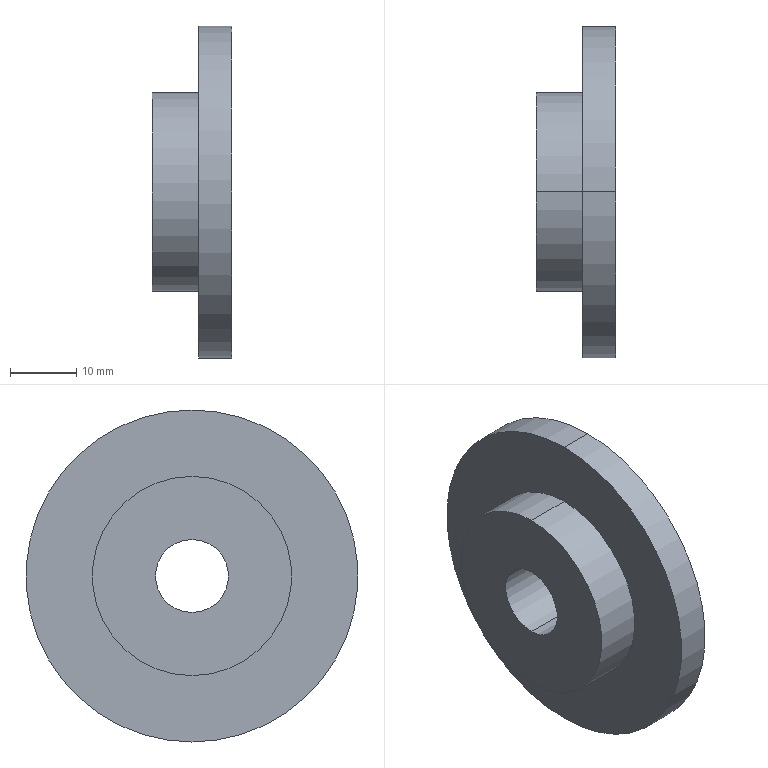Part | SolidWorks | features ICE 1, Revolution 1 | 1 solid | 9 faces | box 12 x 50 x 50 mm | volume 13625 mm3 | cylinder 6 | plane 3 | commonest cylinder face diameters 11 x2 30 x2 50 x2
STEP:
#1=CARTESIAN_POINT('',(0.,0.,5.5));
#2=VERTEX_POINT('',#1);
#3=CARTESIAN_POINT('',(0.,0.,-5.5));
#4=VERTEX_POINT('',#3);
#5=CARTESIAN_POINT('',(0.,0.,0.));
#6=DIRECTION('',(1.,0.,0.));
#7=DIRECTION('',(0.,0.,-1.));
#8=AXIS2_PLACEMENT_3D('',#5,#6,#7);
#9=CIRCLE('',#8,5.5);
#10=EDGE_CURVE('',#2,#4,#9,.T.);
#11=ORIENTED_EDGE('',*,*,#10,.F.);
#12=CARTESIAN_POINT('',(12.,0.,5.5));
#13=VERTEX_POINT('',#12);
#14=CARTESIAN_POINT('',(-5.,0.,5.5));
#15=DIRECTION('',(1.,0.,0.));
#16=VECTOR('',#15,1000.);
#17=LINE('',#14,#16);
#18=EDGE_CURVE('',#2,#13,#17,.T.);
#19=ORIENTED_EDGE('',*,*,#18,.T.);
#20=CARTESIAN_POINT('',(12.,0.,-5.5));
#21=VERTEX_POINT('',#20);
#22=CARTESIAN_POINT('',(12.,0.,0.));
#23=DIRECTION('',(1.,0.,0.));
#24=DIRECTION('',(0.,0.,-1.));
#25=AXIS2_PLACEMENT_3D('',#22,#23,#24);
#26=CIRCLE('',#25,5.5);
#27=EDGE_CURVE('',#13,#21,#26,.T.);
#28=ORIENTED_EDGE('',*,*,#27,.T.);
#29=CARTESIAN_POINT('',(-5.,0.,-5.5));
#30=DIRECTION('',(1.,0.,0.));
#31=VECTOR('',#30,1000.);
#32=LINE('',#29,#31);
#33=EDGE_CURVE('',#4,#21,#32,.T.);
#34=ORIENTED_EDGE('',*,*,#33,.F.);
#35=EDGE_LOOP('',(#11,#19,#28,#34));
#36=FACE_OUTER_BOUND('',#35,.T.);
#37=CARTESIAN_POINT('',(-5.,0.,0.));
#38=DIRECTION('',(1.,0.,0.));
#39=DIRECTION('',(0.,0.,-1.));
#40=AXIS2_PLACEMENT_3D('',#37,#38,#39);
#41=CYLINDRICAL_SURFACE('',#40,5.5);
#42=ADVANCED_FACE('',(#36),#41,.F.);
#43=CARTESIAN_POINT('',(12.,0.,25.));
#44=VERTEX_POINT('',#43);
#45=CARTESIAN_POINT('',(12.,0.,-25.));
#46=VERTEX_POINT('',#45);
#47=CARTESIAN_POINT('',(12.,0.,0.));
#48=DIRECTION('',(-1.,0.,0.));
#49=DIRECTION('',(0.,0.,1.));
#50=AXIS2_PLACEMENT_3D('',#47,#48,#49);
#51=CIRCLE('',#50,25.);
#52=EDGE_CURVE('',#44,#46,#51,.T.);
#53=ORIENTED_EDGE('',*,*,#52,.T.);
#54=CARTESIAN_POINT('',(7.,0.,-25.));
#55=VERTEX_POINT('',#54);
#56=CARTESIAN_POINT('',(0.,0.,-25.));
#57=DIRECTION('',(-1.,0.,0.));
#58=VECTOR('',#57,1000.);
#59=LINE('',#56,#58);
#60=EDGE_CURVE('',#46,#55,#59,.T.);
#61=ORIENTED_EDGE('',*,*,#60,.T.);
#62=CARTESIAN_POINT('',(7.,0.,25.));
#63=VERTEX_POINT('',#62);
#64=CARTESIAN_POINT('',(7.,0.,0.));
#65=DIRECTION('',(-1.,0.,0.));
#66=DIRECTION('',(0.,0.,1.));
#67=AXIS2_PLACEMENT_3D('',#64,#65,#66);
#68=CIRCLE('',#67,25.);
#69=EDGE_CURVE('',#63,#55,#68,.T.);
#70=ORIENTED_EDGE('',*,*,#69,.F.);
#71=CARTESIAN_POINT('',(0.,0.,25.));
#72=DIRECTION('',(-1.,0.,0.));
#73=VECTOR('',#72,1000.);
#74=LINE('',#71,#73);
#75=EDGE_CURVE('',#44,#63,#74,.T.);
#76=ORIENTED_EDGE('',*,*,#75,.F.);
#77=EDGE_LOOP('',(#53,#61,#70,#76));
#78=FACE_OUTER_BOUND('',#77,.T.);
#79=CARTESIAN_POINT('',(0.,0.,0.));
#80=DIRECTION('',(-1.,0.,0.));
#81=DIRECTION('',(0.,0.,1.));
#82=AXIS2_PLACEMENT_3D('',#79,#80,#81);
#83=CYLINDRICAL_SURFACE('',#82,25.);
#84=ADVANCED_FACE('',(#78),#83,.T.);
#85=CARTESIAN_POINT('',(7.,0.,15.));
#86=VERTEX_POINT('',#85);
#87=CARTESIAN_POINT('',(7.,0.,-15.));
#88=VERTEX_POINT('',#87);
#89=CARTESIAN_POINT('',(7.,0.,0.));
#90=DIRECTION('',(-1.,0.,0.));
#91=DIRECTION('',(0.,0.,1.));
#92=AXIS2_PLACEMENT_3D('',#89,#90,#91);
#93=CIRCLE('',#92,15.);
#94=EDGE_CURVE('',#86,#88,#93,.T.);
#95=ORIENTED_EDGE('',*,*,#94,.T.);
#96=CARTESIAN_POINT('',(0.,0.,-15.));
#97=VERTEX_POINT('',#96);
#98=CARTESIAN_POINT('',(0.,0.,-15.));
#99=DIRECTION('',(-1.,0.,0.));
#100=VECTOR('',#99,1000.);
#101=LINE('',#98,#100);
#102=EDGE_CURVE('',#88,#97,#101,.T.);
#103=ORIENTED_EDGE('',*,*,#102,.T.);
#104=CARTESIAN_POINT('',(0.,0.,15.));
#105=VERTEX_POINT('',#104);
#106=CARTESIAN_POINT('',(0.,0.,0.));
#107=DIRECTION('',(-1.,0.,0.));
#108=DIRECTION('',(0.,0.,1.));
#109=AXIS2_PLACEMENT_3D('',#106,#107,#108);
#110=CIRCLE('',#109,15.);
#111=EDGE_CURVE('',#105,#97,#110,.T.);
#112=ORIENTED_EDGE('',*,*,#111,.F.);
#113=CARTESIAN_POINT('',(0.,0.,15.));
#114=DIRECTION('',(-1.,0.,0.));
#115=VECTOR('',#114,1000.);
#116=LINE('',#113,#115);
#117=EDGE_CURVE('',#86,#105,#116,.T.);
#118=ORIENTED_EDGE('',*,*,#117,.F.);
#119=EDGE_LOOP('',(#95,#103,#112,#118));
#120=FACE_OUTER_BOUND('',#119,.T.);
#121=CARTESIAN_POINT('',(0.,0.,0.));
#122=DIRECTION('',(-1.,0.,0.));
#123=DIRECTION('',(0.,0.,1.));
#124=AXIS2_PLACEMENT_3D('',#121,#122,#123);
#125=CYLINDRICAL_SURFACE('',#124,15.);
#126=ADVANCED_FACE('',(#120),#125,.T.);
#127=CARTESIAN_POINT('',(0.,0.,0.));
#128=DIRECTION('',(1.,0.,0.));
#129=DIRECTION('',(0.,0.,-1.));
#130=AXIS2_PLACEMENT_3D('',#127,#128,#129);
#131=CIRCLE('',#130,5.5);
#132=EDGE_CURVE('',#4,#2,#131,.T.);
#133=ORIENTED_EDGE('',*,*,#132,.T.);
#134=ORIENTED_EDGE('',*,*,#10,.T.);
#135=EDGE_LOOP('',(#133,#134));
#136=FACE_BOUND('',#135,.T.);
#137=ORIENTED_EDGE('',*,*,#111,.T.);
#138=CARTESIAN_POINT('',(0.,0.,0.));
#139=DIRECTION('',(-1.,0.,0.));
#140=DIRECTION('',(0.,0.,1.));
#141=AXIS2_PLACEMENT_3D('',#138,#139,#140);
#142=CIRCLE('',#141,15.);
#143=EDGE_CURVE('',#97,#105,#142,.T.);
#144=ORIENTED_EDGE('',*,*,#143,.T.);
#145=EDGE_LOOP('',(#137,#144));
#146=FACE_OUTER_BOUND('',#145,.T.);
#147=CARTESIAN_POINT('',(0.,0.,0.));
#148=DIRECTION('',(1.,0.,0.));
#149=DIRECTION('',(0.,0.,-1.));
#150=AXIS2_PLACEMENT_3D('',#147,#148,#149);
#151=PLANE('',#150);
#152=ADVANCED_FACE('',(#136,#146),#151,.F.);
#153=ORIENTED_EDGE('',*,*,#102,.F.);
#154=CARTESIAN_POINT('',(7.,0.,0.));
#155=DIRECTION('',(-1.,0.,0.));
#156=DIRECTION('',(0.,0.,1.));
#157=AXIS2_PLACEMENT_3D('',#154,#155,#156);
#158=CIRCLE('',#157,15.);
#159=EDGE_CURVE('',#88,#86,#158,.T.);
#160=ORIENTED_EDGE('',*,*,#159,.T.);
#161=ORIENTED_EDGE('',*,*,#117,.T.);
#162=ORIENTED_EDGE('',*,*,#143,.F.);
#163=EDGE_LOOP('',(#153,#160,#161,#162));
#164=FACE_OUTER_BOUND('',#163,.T.);
#165=CARTESIAN_POINT('',(0.,0.,0.));
#166=DIRECTION('',(-1.,0.,0.));
#167=DIRECTION('',(0.,0.,1.));
#168=AXIS2_PLACEMENT_3D('',#165,#166,#167);
#169=CYLINDRICAL_SURFACE('',#168,15.);
#170=ADVANCED_FACE('',(#164),#169,.T.);
#171=ORIENTED_EDGE('',*,*,#94,.F.);
#172=ORIENTED_EDGE('',*,*,#159,.F.);
#173=EDGE_LOOP('',(#171,#172));
#174=FACE_BOUND('',#173,.T.);
#175=ORIENTED_EDGE('',*,*,#69,.T.);
#176=CARTESIAN_POINT('',(7.,0.,0.));
#177=DIRECTION('',(-1.,0.,0.));
#178=DIRECTION('',(0.,0.,1.));
#179=AXIS2_PLACEMENT_3D('',#176,#177,#178);
#180=CIRCLE('',#179,25.);
#181=EDGE_CURVE('',#55,#63,#180,.T.);
#182=ORIENTED_EDGE('',*,*,#181,.T.);
#183=EDGE_LOOP('',(#175,#182));
#184=FACE_OUTER_BOUND('',#183,.T.);
#185=CARTESIAN_POINT('',(7.,15.,0.));
#186=DIRECTION('',(1.,0.,0.));
#187=DIRECTION('',(0.,0.,-1.));
#188=AXIS2_PLACEMENT_3D('',#185,#186,#187);
#189=PLANE('',#188);
#190=ADVANCED_FACE('',(#174,#184),#189,.F.);
#191=ORIENTED_EDGE('',*,*,#60,.F.);
#192=CARTESIAN_POINT('',(12.,0.,0.));
#193=DIRECTION('',(-1.,0.,0.));
#194=DIRECTION('',(0.,0.,1.));
#195=AXIS2_PLACEMENT_3D('',#192,#193,#194);
#196=CIRCLE('',#195,25.);
#197=EDGE_CURVE('',#46,#44,#196,.T.);
#198=ORIENTED_EDGE('',*,*,#197,.T.);
#199=ORIENTED_EDGE('',*,*,#75,.T.);
#200=ORIENTED_EDGE('',*,*,#181,.F.);
#201=EDGE_LOOP('',(#191,#198,#199,#200));
#202=FACE_OUTER_BOUND('',#201,.T.);
#203=CARTESIAN_POINT('',(0.,0.,0.));
#204=DIRECTION('',(-1.,0.,0.));
#205=DIRECTION('',(0.,0.,1.));
#206=AXIS2_PLACEMENT_3D('',#203,#204,#205);
#207=CYLINDRICAL_SURFACE('',#206,25.);
#208=ADVANCED_FACE('',(#202),#207,.T.);
#209=CARTESIAN_POINT('',(12.,0.,0.));
#210=DIRECTION('',(1.,0.,0.));
#211=DIRECTION('',(0.,0.,-1.));
#212=AXIS2_PLACEMENT_3D('',#209,#210,#211);
#213=CIRCLE('',#212,5.5);
#214=EDGE_CURVE('',#21,#13,#213,.T.);
#215=ORIENTED_EDGE('',*,*,#214,.F.);
#216=ORIENTED_EDGE('',*,*,#27,.F.);
#217=EDGE_LOOP('',(#215,#216));
#218=FACE_BOUND('',#217,.T.);
#219=ORIENTED_EDGE('',*,*,#52,.F.);
#220=ORIENTED_EDGE('',*,*,#197,.F.);
#221=EDGE_LOOP('',(#219,#220));
#222=FACE_OUTER_BOUND('',#221,.T.);
#223=CARTESIAN_POINT('',(12.,25.,0.));
#224=DIRECTION('',(-1.,0.,0.));
#225=DIRECTION('',(0.,0.,1.));
#226=AXIS2_PLACEMENT_3D('',#223,#224,#225);
#227=PLANE('',#226);
#228=ADVANCED_FACE('',(#218,#222),#227,.F.);
#229=ORIENTED_EDGE('',*,*,#18,.F.);
#230=ORIENTED_EDGE('',*,*,#132,.F.);
#231=ORIENTED_EDGE('',*,*,#33,.T.);
#232=ORIENTED_EDGE('',*,*,#214,.T.);
#233=EDGE_LOOP('',(#229,#230,#231,#232));
#234=FACE_OUTER_BOUND('',#233,.T.);
#235=CARTESIAN_POINT('',(-5.,0.,0.));
#236=DIRECTION('',(1.,0.,0.));
#237=DIRECTION('',(0.,0.,-1.));
#238=AXIS2_PLACEMENT_3D('',#235,#236,#237);
#239=CYLINDRICAL_SURFACE('',#238,5.5);
#240=ADVANCED_FACE('',(#234),#239,.F.);
#241=CLOSED_SHELL('',(#42,#84,#126,#152,#170,#190,#208,#228,#240));
#242=MANIFOLD_SOLID_BREP('',#241);
#243=CARTESIAN_POINT('',(0.,0.,0.));
#244=DIRECTION('',(0.,0.,1.));
#245=DIRECTION('',(1.,0.,0.));
#246=AXIS2_PLACEMENT_3D('',#243,#244,#245);
#247=(LENGTH_UNIT()NAMED_UNIT(*)SI_UNIT(.MILLI.,.METRE.));
#248=UNCERTAINTY_MEASURE_WITH_UNIT(LENGTH_MEASURE(0.00001),#247,'','');
#249=(NAMED_UNIT(*)PLANE_ANGLE_UNIT()SI_UNIT($,.RADIAN.));
#250=(NAMED_UNIT(*)SI_UNIT($,.STERADIAN.)SOLID_ANGLE_UNIT());
#251=(GEOMETRIC_REPRESENTATION_CONTEXT(3)GLOBAL_UNCERTAINTY_ASSIGNED_CONTEXT((#248))GLOBAL_UNIT_ASSIGNED_CONTEXT((#247,#249,#250))REPRESENTATION_CONTEXT('',''));
#252=ADVANCED_BREP_SHAPE_REPRESENTATION('',(#242,#246),#251);